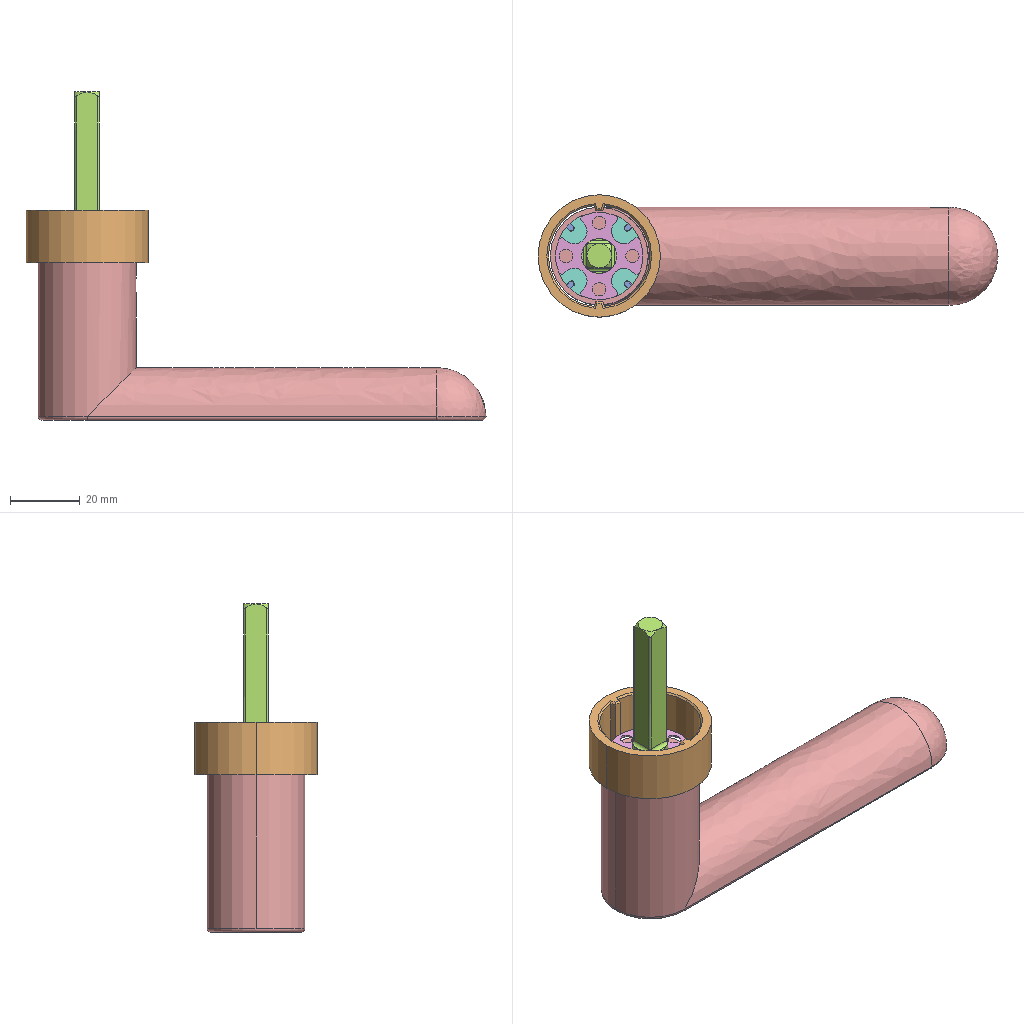Assembly | SolidWorks | 6 different items | 6 placed | box 132 x 35 x 94 mm
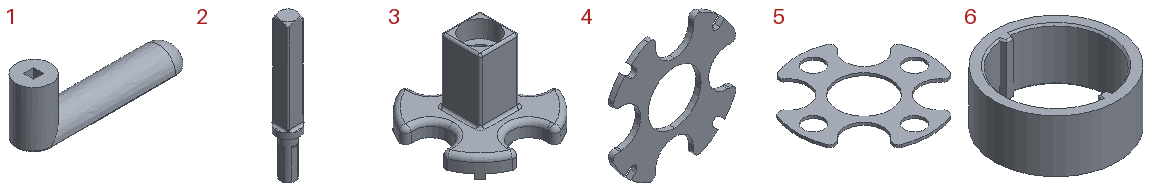Parts list (item | quantity | size | volume | features):
1 | x1 | 128.025 x 28 x 45 mm | 59416 mm3 | features ICE 5, Cut 2, Blend 1, Extrusion 1, Fillet 1, HoleWzd 1, NetBlend 1
2 | x1 | 10 x 10 x 62 mm | 2691 mm3 | features Fillet 3, ICE 3, Extrusion 1, HoleWzd 1, RevCut 1
3 | x1 | 23.109 x 23.109 x 18.5 mm | 1457 mm3 | features ICE 6, Fillet 3, Chamfer 1, Extrusion 1, RevCut 1
4 | x1 | 23.109 x 1 x 23.109 mm | 247.856 mm3 | features Extrusion 1
5 | x1 | 25 x 25 x 0.5 mm | 107.561 mm3 | features Extrusion 1
6 | x1 | 35 x 35 x 15 mm | 4612 mm3 | features Chamfer 1, Extrusion 1, ICE 1
Mates (type | each side: item.copy, entity, surface, feature):
ProfileCenter | 3.1 face plane Boss-Extrude2 | 1.1 face plane Cut-Extrude4
Concentric | 3.1 face cylinder Boss-Extrude3 | 2.1 face cylinder Boss-Extrude3
Parallel | 3.1 face plane Boss-Extrude3 | 2.1 face plane Cut-Extrude2
Coincident | 3.1 face plane Boss-Extrude3 | 2.1 face plane Boss-Extrude1
Concentric | 3.1 face cylinder Boss-Extrude3 | 5.1 face cylinder Boss-Extrude1
Concentric | 3.1 face cylinder Boss-Extrude3 | 4.1 face cylinder Boss-Extrude1
Parallel | 3.1 face plane Boss-Extrude4 | 4.1 face plane Boss-Extrude1
Coincident | 3.1 face plane Boss-Extrude1 | 4.1 face plane Boss-Extrude1
Coincident | 5.1 face plane Boss-Extrude1 | 4.1 face plane Boss-Extrude1
Parallel | 2.1 face plane Boss-Extrude2 | 5.1 plane
Concentric | 3.1 face cylinder Boss-Extrude1 | 6.1 face cylinder Boss-Extrude1
Parallel | 2.1 face plane Boss-Extrude2 | 6.1 plane
Coincident | 1.1 face plane Boss-Extrude1 | 6.1 face plane Boss-Extrude1